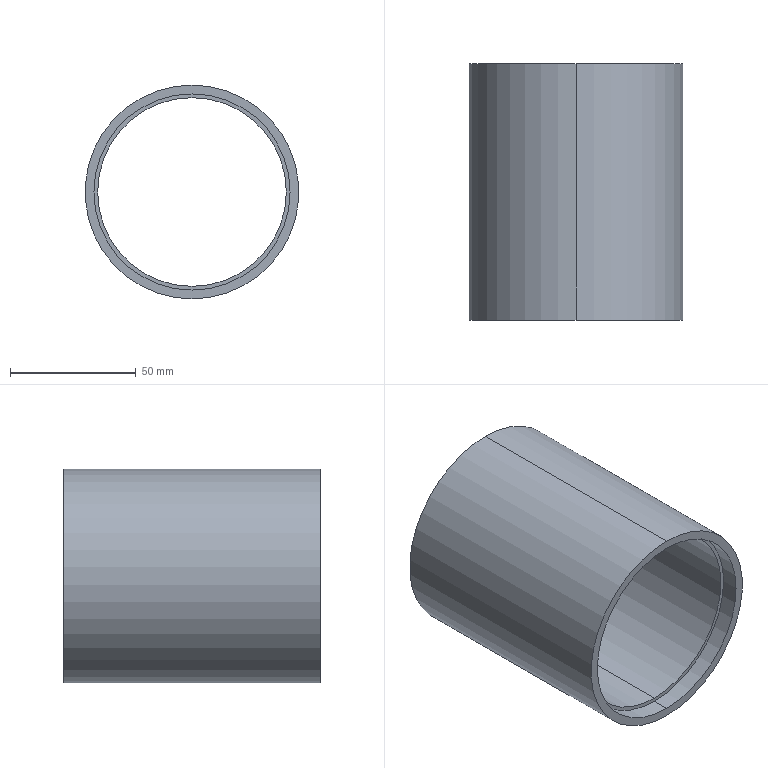Part | STEP file | 0229_Work-A | 1 solid | 11 faces | box 85 x 102 x 85 mm | volume 125379 mm3 | cylinder 6 | plane 3 | cone 2 | commonest cylinder face diameters 75 x2 78 x2 85 x2
STEP:
#1=CARTESIAN_POINT('',(0.,0.,0.));
#2=DIRECTION('',(0.,0.,1.));
#3=DIRECTION('',(1.,0.,0.));
#4=AXIS2_PLACEMENT_3D('',#1,#2,#3);
#5=CARTESIAN_POINT('',(0.,100.,37.5));
#6=VERTEX_POINT('',#5);
#7=CARTESIAN_POINT('',(0.,102.,38.655));
#8=VERTEX_POINT('',#7);
#9=CARTESIAN_POINT('',(0.,102.,38.655));
#10=DIRECTION('',(0.,0.866,0.5));
#11=VECTOR('',#10,1.);
#12=LINE('',#9,#11);
#13=CARTESIAN_POINT('',(0.,102.,0.));
#14=DIRECTION('',(0.,1.,0.));
#15=DIRECTION('',(0.,0.,1.));
#16=AXIS2_PLACEMENT_3D('',#13,#14,#15);
#17=CONICAL_SURFACE('',#16,38.655,0.5236);
#18=CARTESIAN_POINT('',(6.283,0.));
#19=DIRECTION('',(0.,1.));
#20=VECTOR('',#19,1.);
#21=LINE('',#18,#20);
#22=(GEOMETRIC_REPRESENTATION_CONTEXT(2)PARAMETRIC_REPRESENTATION_CONTEXT()REPRESENTATION_CONTEXT('',''));
#23=DEFINITIONAL_REPRESENTATION('',(#21),#22);
#24=PCURVE('',#17,#23);
#25=CARTESIAN_POINT('',(0.,102.,0.));
#26=DIRECTION('',(0.,1.,0.));
#27=DIRECTION('',(0.,0.,1.));
#28=AXIS2_PLACEMENT_3D('',#25,#26,#27);
#29=CONICAL_SURFACE('',#28,38.655,0.5236);
#30=CARTESIAN_POINT('',(0.,0.));
#31=DIRECTION('',(0.,1.));
#32=VECTOR('',#31,1.);
#33=LINE('',#30,#32);
#34=(GEOMETRIC_REPRESENTATION_CONTEXT(2)PARAMETRIC_REPRESENTATION_CONTEXT()REPRESENTATION_CONTEXT('',''));
#35=DEFINITIONAL_REPRESENTATION('',(#33),#34);
#36=PCURVE('',#29,#35);
#37=SURFACE_CURVE('',#12,(#24,#36),.PCURVE_S1.);
#38=EDGE_CURVE('',#6,#8,#37,.T.);
#39=ORIENTED_EDGE('',*,*,#38,.T.);
#40=CARTESIAN_POINT('',(0.,102.,-38.655));
#41=VERTEX_POINT('',#40);
#42=CARTESIAN_POINT('',(0.,102.,0.));
#43=DIRECTION('',(0.,-1.,0.));
#44=DIRECTION('',(0.,0.,-1.));
#45=AXIS2_PLACEMENT_3D('',#42,#43,#44);
#46=CIRCLE('',#45,38.655);
#47=CARTESIAN_POINT('',(9.425,0.));
#48=DIRECTION('',(-1.,0.));
#49=VECTOR('',#48,1.);
#50=LINE('',#47,#49);
#51=(GEOMETRIC_REPRESENTATION_CONTEXT(2)PARAMETRIC_REPRESENTATION_CONTEXT()REPRESENTATION_CONTEXT('',''));
#52=DEFINITIONAL_REPRESENTATION('',(#50),#51);
#53=PCURVE('',#17,#52);
#54=CARTESIAN_POINT('',(0.,102.,0.));
#55=DIRECTION('',(0.,-1.,0.));
#56=DIRECTION('',(0.,0.,-1.));
#57=AXIS2_PLACEMENT_3D('',#54,#55,#56);
#58=PLANE('',#57);
#59=CARTESIAN_POINT('',(0.,0.));
#60=DIRECTION('',(1.,0.));
#61=AXIS2_PLACEMENT_2D('',#59,#60);
#62=CIRCLE('',#61,38.655);
#63=(GEOMETRIC_REPRESENTATION_CONTEXT(2)PARAMETRIC_REPRESENTATION_CONTEXT()REPRESENTATION_CONTEXT('',''));
#64=DEFINITIONAL_REPRESENTATION('',(#62),#63);
#65=PCURVE('',#58,#64);
#66=SURFACE_CURVE('',#46,(#53,#65),.PCURVE_S1.);
#67=EDGE_CURVE('',#8,#41,#66,.T.);
#68=ORIENTED_EDGE('',*,*,#67,.T.);
#69=CARTESIAN_POINT('',(0.,100.,-37.5));
#70=VERTEX_POINT('',#69);
#71=CARTESIAN_POINT('',(0.,102.,-38.655));
#72=DIRECTION('',(0.,0.866,-0.5));
#73=VECTOR('',#72,1.);
#74=LINE('',#71,#73);
#75=CARTESIAN_POINT('',(3.142,0.));
#76=DIRECTION('',(0.,1.));
#77=VECTOR('',#76,1.);
#78=LINE('',#75,#77);
#79=(GEOMETRIC_REPRESENTATION_CONTEXT(2)PARAMETRIC_REPRESENTATION_CONTEXT()REPRESENTATION_CONTEXT('',''));
#80=DEFINITIONAL_REPRESENTATION('',(#78),#79);
#81=PCURVE('',#17,#80);
#82=CARTESIAN_POINT('',(3.142,0.));
#83=DIRECTION('',(0.,1.));
#84=VECTOR('',#83,1.);
#85=LINE('',#82,#84);
#86=(GEOMETRIC_REPRESENTATION_CONTEXT(2)PARAMETRIC_REPRESENTATION_CONTEXT()REPRESENTATION_CONTEXT('',''));
#87=DEFINITIONAL_REPRESENTATION('',(#85),#86);
#88=PCURVE('',#29,#87);
#89=SURFACE_CURVE('',#74,(#81,#88),.PCURVE_S1.);
#90=EDGE_CURVE('',#70,#41,#89,.T.);
#91=ORIENTED_EDGE('',*,*,#90,.F.);
#92=CARTESIAN_POINT('',(0.,100.,0.));
#93=DIRECTION('',(0.,1.,0.));
#94=DIRECTION('',(0.,0.,-1.));
#95=AXIS2_PLACEMENT_3D('',#92,#93,#94);
#96=CIRCLE('',#95,37.5);
#97=CARTESIAN_POINT('',(3.142,-2.));
#98=DIRECTION('',(1.,0.));
#99=VECTOR('',#98,1.);
#100=LINE('',#97,#99);
#101=(GEOMETRIC_REPRESENTATION_CONTEXT(2)PARAMETRIC_REPRESENTATION_CONTEXT()REPRESENTATION_CONTEXT('',''));
#102=DEFINITIONAL_REPRESENTATION('',(#100),#101);
#103=PCURVE('',#17,#102);
#104=CARTESIAN_POINT('',(0.,-11.457,0.));
#105=DIRECTION('',(0.,-1.,0.));
#106=DIRECTION('',(0.,0.,-1.));
#107=AXIS2_PLACEMENT_3D('',#104,#105,#106);
#108=CYLINDRICAL_SURFACE('',#107,37.5);
#109=CARTESIAN_POINT('',(6.283,-111.457));
#110=DIRECTION('',(-1.,0.));
#111=VECTOR('',#110,1.);
#112=LINE('',#109,#111);
#113=(GEOMETRIC_REPRESENTATION_CONTEXT(2)PARAMETRIC_REPRESENTATION_CONTEXT()REPRESENTATION_CONTEXT('',''));
#114=DEFINITIONAL_REPRESENTATION('',(#112),#113);
#115=PCURVE('',#108,#114);
#116=SURFACE_CURVE('',#96,(#103,#115),.PCURVE_S1.);
#117=EDGE_CURVE('',#70,#6,#116,.T.);
#118=ORIENTED_EDGE('',*,*,#117,.T.);
#119=EDGE_LOOP('',(#39,#68,#91,#118));
#120=FACE_BOUND('',#119,.F.);
#121=ADVANCED_FACE('',(#120),#17,.F.);
#122=CARTESIAN_POINT('',(0.,7.,-39.));
#123=VERTEX_POINT('',#122);
#124=CARTESIAN_POINT('',(0.,0.,-39.));
#125=VERTEX_POINT('',#124);
#126=CARTESIAN_POINT('',(0.,-11.457,-39.));
#127=DIRECTION('',(0.,-1.,0.));
#128=VECTOR('',#127,1.);
#129=LINE('',#126,#128);
#130=CARTESIAN_POINT('',(0.,-11.457,0.));
#131=DIRECTION('',(0.,-1.,0.));
#132=DIRECTION('',(0.,0.,-1.));
#133=AXIS2_PLACEMENT_3D('',#130,#131,#132);
#134=CYLINDRICAL_SURFACE('',#133,39.);
#135=CARTESIAN_POINT('',(6.283,0.));
#136=DIRECTION('',(0.,1.));
#137=VECTOR('',#136,1.);
#138=LINE('',#135,#137);
#139=(GEOMETRIC_REPRESENTATION_CONTEXT(2)PARAMETRIC_REPRESENTATION_CONTEXT()REPRESENTATION_CONTEXT('',''));
#140=DEFINITIONAL_REPRESENTATION('',(#138),#139);
#141=PCURVE('',#134,#140);
#142=CARTESIAN_POINT('',(0.,-11.457,0.));
#143=DIRECTION('',(0.,-1.,0.));
#144=DIRECTION('',(0.,0.,-1.));
#145=AXIS2_PLACEMENT_3D('',#142,#143,#144);
#146=CYLINDRICAL_SURFACE('',#145,39.);
#147=CARTESIAN_POINT('',(0.,0.));
#148=DIRECTION('',(0.,1.));
#149=VECTOR('',#148,1.);
#150=LINE('',#147,#149);
#151=(GEOMETRIC_REPRESENTATION_CONTEXT(2)PARAMETRIC_REPRESENTATION_CONTEXT()REPRESENTATION_CONTEXT('',''));
#152=DEFINITIONAL_REPRESENTATION('',(#150),#151);
#153=PCURVE('',#146,#152);
#154=SURFACE_CURVE('',#129,(#141,#153),.PCURVE_S1.);
#155=EDGE_CURVE('',#123,#125,#154,.T.);
#156=ORIENTED_EDGE('',*,*,#155,.T.);
#157=CARTESIAN_POINT('',(0.,0.,39.));
#158=VERTEX_POINT('',#157);
#159=CARTESIAN_POINT('',(0.,0.,0.));
#160=DIRECTION('',(0.,-1.,0.));
#161=DIRECTION('',(0.,0.,-1.));
#162=AXIS2_PLACEMENT_3D('',#159,#160,#161);
#163=CIRCLE('',#162,39.);
#164=CARTESIAN_POINT('',(0.,-11.457));
#165=DIRECTION('',(1.,0.));
#166=VECTOR('',#165,1.);
#167=LINE('',#164,#166);
#168=(GEOMETRIC_REPRESENTATION_CONTEXT(2)PARAMETRIC_REPRESENTATION_CONTEXT()REPRESENTATION_CONTEXT('',''));
#169=DEFINITIONAL_REPRESENTATION('',(#167),#168);
#170=PCURVE('',#134,#169);
#171=CARTESIAN_POINT('',(0.,0.,0.));
#172=DIRECTION('',(0.,1.,0.));
#173=DIRECTION('',(0.,0.,1.));
#174=AXIS2_PLACEMENT_3D('',#171,#172,#173);
#175=PLANE('',#174);
#176=CARTESIAN_POINT('',(-39.,0.));
#177=CARTESIAN_POINT('',(-39.,67.55));
#178=CARTESIAN_POINT('',(19.5,33.775));
#179=CARTESIAN_POINT('',(78.,0.));
#180=CARTESIAN_POINT('',(19.5,-33.775));
#181=CARTESIAN_POINT('',(-39.,-67.55));
#182=CARTESIAN_POINT('',(-39.,0.));
#183=(BOUNDED_CURVE()B_SPLINE_CURVE(2,(#176,#177,#178,#179,#180,#181,#182),.UNSPECIFIED.,.T.,.F.)B_SPLINE_CURVE_WITH_KNOTS((1,2,2,2,2,1),(-2.094,0.,2.094,4.189,6.283,8.378),.UNSPECIFIED.)CURVE()GEOMETRIC_REPRESENTATION_ITEM()RATIONAL_B_SPLINE_CURVE((1.,0.5,1.,0.5,1.,0.5,1.))REPRESENTATION_ITEM(''));
#184=(GEOMETRIC_REPRESENTATION_CONTEXT(2)PARAMETRIC_REPRESENTATION_CONTEXT()REPRESENTATION_CONTEXT('',''));
#185=DEFINITIONAL_REPRESENTATION('',(#183),#184);
#186=PCURVE('',#175,#185);
#187=SURFACE_CURVE('',#163,(#170,#186),.PCURVE_S1.);
#188=EDGE_CURVE('',#158,#125,#187,.T.);
#189=ORIENTED_EDGE('',*,*,#188,.F.);
#190=CARTESIAN_POINT('',(0.,7.,39.));
#191=VERTEX_POINT('',#190);
#192=CARTESIAN_POINT('',(0.,-11.457,39.));
#193=DIRECTION('',(0.,-1.,0.));
#194=VECTOR('',#193,1.);
#195=LINE('',#192,#194);
#196=CARTESIAN_POINT('',(3.142,0.));
#197=DIRECTION('',(0.,1.));
#198=VECTOR('',#197,1.);
#199=LINE('',#196,#198);
#200=(GEOMETRIC_REPRESENTATION_CONTEXT(2)PARAMETRIC_REPRESENTATION_CONTEXT()REPRESENTATION_CONTEXT('',''));
#201=DEFINITIONAL_REPRESENTATION('',(#199),#200);
#202=PCURVE('',#134,#201);
#203=CARTESIAN_POINT('',(3.142,0.));
#204=DIRECTION('',(0.,1.));
#205=VECTOR('',#204,1.);
#206=LINE('',#203,#205);
#207=(GEOMETRIC_REPRESENTATION_CONTEXT(2)PARAMETRIC_REPRESENTATION_CONTEXT()REPRESENTATION_CONTEXT('',''));
#208=DEFINITIONAL_REPRESENTATION('',(#206),#207);
#209=PCURVE('',#146,#208);
#210=SURFACE_CURVE('',#195,(#202,#209),.PCURVE_S1.);
#211=EDGE_CURVE('',#191,#158,#210,.T.);
#212=ORIENTED_EDGE('',*,*,#211,.F.);
#213=CARTESIAN_POINT('',(0.,7.,0.));
#214=DIRECTION('',(0.,-1.,0.));
#215=DIRECTION('',(0.,0.,-1.));
#216=AXIS2_PLACEMENT_3D('',#213,#214,#215);
#217=CIRCLE('',#216,39.);
#218=CARTESIAN_POINT('',(0.,-18.457));
#219=DIRECTION('',(1.,0.));
#220=VECTOR('',#219,1.);
#221=LINE('',#218,#220);
#222=(GEOMETRIC_REPRESENTATION_CONTEXT(2)PARAMETRIC_REPRESENTATION_CONTEXT()REPRESENTATION_CONTEXT('',''));
#223=DEFINITIONAL_REPRESENTATION('',(#221),#222);
#224=PCURVE('',#134,#223);
#225=CARTESIAN_POINT('',(-37.5,7.,0.));
#226=DIRECTION('',(0.,-1.,0.));
#227=DIRECTION('',(0.,0.,-1.));
#228=AXIS2_PLACEMENT_3D('',#225,#226,#227);
#229=PLANE('',#228);
#230=CARTESIAN_POINT('',(0.,37.5));
#231=DIRECTION('',(1.,0.));
#232=AXIS2_PLACEMENT_2D('',#230,#231);
#233=CIRCLE('',#232,39.);
#234=(GEOMETRIC_REPRESENTATION_CONTEXT(2)PARAMETRIC_REPRESENTATION_CONTEXT()REPRESENTATION_CONTEXT('',''));
#235=DEFINITIONAL_REPRESENTATION('',(#233),#234);
#236=PCURVE('',#229,#235);
#237=SURFACE_CURVE('',#217,(#224,#236),.PCURVE_S1.);
#238=EDGE_CURVE('',#191,#123,#237,.T.);
#239=ORIENTED_EDGE('',*,*,#238,.T.);
#240=EDGE_LOOP('',(#156,#189,#212,#239));
#241=FACE_BOUND('',#240,.F.);
#242=ADVANCED_FACE('',(#241),#134,.F.);
#243=CARTESIAN_POINT('',(0.,7.,-37.5));
#244=VERTEX_POINT('',#243);
#245=CARTESIAN_POINT('',(0.,-11.457,-37.5));
#246=DIRECTION('',(0.,-1.,0.));
#247=VECTOR('',#246,1.);
#248=LINE('',#245,#247);
#249=CARTESIAN_POINT('',(6.283,0.));
#250=DIRECTION('',(0.,1.));
#251=VECTOR('',#250,1.);
#252=LINE('',#249,#251);
#253=(GEOMETRIC_REPRESENTATION_CONTEXT(2)PARAMETRIC_REPRESENTATION_CONTEXT()REPRESENTATION_CONTEXT('',''));
#254=DEFINITIONAL_REPRESENTATION('',(#252),#253);
#255=PCURVE('',#108,#254);
#256=CARTESIAN_POINT('',(0.,-11.457,0.));
#257=DIRECTION('',(0.,-1.,0.));
#258=DIRECTION('',(0.,0.,-1.));
#259=AXIS2_PLACEMENT_3D('',#256,#257,#258);
#260=CYLINDRICAL_SURFACE('',#259,37.5);
#261=CARTESIAN_POINT('',(0.,0.));
#262=DIRECTION('',(0.,1.));
#263=VECTOR('',#262,1.);
#264=LINE('',#261,#263);
#265=(GEOMETRIC_REPRESENTATION_CONTEXT(2)PARAMETRIC_REPRESENTATION_CONTEXT()REPRESENTATION_CONTEXT('',''));
#266=DEFINITIONAL_REPRESENTATION('',(#264),#265);
#267=PCURVE('',#260,#266);
#268=SURFACE_CURVE('',#248,(#255,#267),.PCURVE_S1.);
#269=EDGE_CURVE('',#70,#244,#268,.T.);
#270=ORIENTED_EDGE('',*,*,#269,.T.);
#271=CARTESIAN_POINT('',(0.,7.,37.5));
#272=VERTEX_POINT('',#271);
#273=CARTESIAN_POINT('',(0.,7.,0.));
#274=DIRECTION('',(0.,-1.,0.));
#275=DIRECTION('',(0.,0.,-1.));
#276=AXIS2_PLACEMENT_3D('',#273,#274,#275);
#277=CIRCLE('',#276,37.5);
#278=CARTESIAN_POINT('',(0.,-18.457));
#279=DIRECTION('',(1.,0.));
#280=VECTOR('',#279,1.);
#281=LINE('',#278,#280);
#282=(GEOMETRIC_REPRESENTATION_CONTEXT(2)PARAMETRIC_REPRESENTATION_CONTEXT()REPRESENTATION_CONTEXT('',''));
#283=DEFINITIONAL_REPRESENTATION('',(#281),#282);
#284=PCURVE('',#108,#283);
#285=CARTESIAN_POINT('',(0.,37.5));
#286=DIRECTION('',(1.,0.));
#287=AXIS2_PLACEMENT_2D('',#285,#286);
#288=CIRCLE('',#287,37.5);
#289=(GEOMETRIC_REPRESENTATION_CONTEXT(2)PARAMETRIC_REPRESENTATION_CONTEXT()REPRESENTATION_CONTEXT('',''));
#290=DEFINITIONAL_REPRESENTATION('',(#288),#289);
#291=PCURVE('',#229,#290);
#292=SURFACE_CURVE('',#277,(#284,#291),.PCURVE_S1.);
#293=EDGE_CURVE('',#272,#244,#292,.T.);
#294=ORIENTED_EDGE('',*,*,#293,.F.);
#295=CARTESIAN_POINT('',(0.,-11.457,37.5));
#296=DIRECTION('',(0.,-1.,0.));
#297=VECTOR('',#296,1.);
#298=LINE('',#295,#297);
#299=CARTESIAN_POINT('',(3.142,0.));
#300=DIRECTION('',(0.,1.));
#301=VECTOR('',#300,1.);
#302=LINE('',#299,#301);
#303=(GEOMETRIC_REPRESENTATION_CONTEXT(2)PARAMETRIC_REPRESENTATION_CONTEXT()REPRESENTATION_CONTEXT('',''));
#304=DEFINITIONAL_REPRESENTATION('',(#302),#303);
#305=PCURVE('',#108,#304);
#306=CARTESIAN_POINT('',(3.142,0.));
#307=DIRECTION('',(0.,1.));
#308=VECTOR('',#307,1.);
#309=LINE('',#306,#308);
#310=(GEOMETRIC_REPRESENTATION_CONTEXT(2)PARAMETRIC_REPRESENTATION_CONTEXT()REPRESENTATION_CONTEXT('',''));
#311=DEFINITIONAL_REPRESENTATION('',(#309),#310);
#312=PCURVE('',#260,#311);
#313=SURFACE_CURVE('',#298,(#305,#312),.PCURVE_S1.);
#314=EDGE_CURVE('',#6,#272,#313,.T.);
#315=ORIENTED_EDGE('',*,*,#314,.F.);
#316=ORIENTED_EDGE('',*,*,#117,.F.);
#317=EDGE_LOOP('',(#270,#294,#315,#316));
#318=FACE_BOUND('',#317,.F.);
#319=ADVANCED_FACE('',(#318),#108,.F.);
#320=CARTESIAN_POINT('',(0.,102.,-42.5));
#321=VERTEX_POINT('',#320);
#322=CARTESIAN_POINT('',(0.,102.,42.5));
#323=VERTEX_POINT('',#322);
#324=CARTESIAN_POINT('',(0.,102.,0.));
#325=DIRECTION('',(0.,-1.,0.));
#326=DIRECTION('',(0.,0.,-1.));
#327=AXIS2_PLACEMENT_3D('',#324,#325,#326);
#328=CIRCLE('',#327,42.5);
#329=CARTESIAN_POINT('',(0.,-9.836,0.));
#330=DIRECTION('',(0.,-1.,0.));
#331=DIRECTION('',(0.,0.,-1.));
#332=AXIS2_PLACEMENT_3D('',#329,#330,#331);
#333=CYLINDRICAL_SURFACE('',#332,42.5);
#334=CARTESIAN_POINT('',(0.,-111.836));
#335=DIRECTION('',(1.,0.));
#336=VECTOR('',#335,1.);
#337=LINE('',#334,#336);
#338=(GEOMETRIC_REPRESENTATION_CONTEXT(2)PARAMETRIC_REPRESENTATION_CONTEXT()REPRESENTATION_CONTEXT('',''));
#339=DEFINITIONAL_REPRESENTATION('',(#337),#338);
#340=PCURVE('',#333,#339);
#341=CARTESIAN_POINT('',(0.,0.));
#342=DIRECTION('',(1.,0.));
#343=AXIS2_PLACEMENT_2D('',#341,#342);
#344=CIRCLE('',#343,42.5);
#345=(GEOMETRIC_REPRESENTATION_CONTEXT(2)PARAMETRIC_REPRESENTATION_CONTEXT()REPRESENTATION_CONTEXT('',''));
#346=DEFINITIONAL_REPRESENTATION('',(#344),#345);
#347=PCURVE('',#58,#346);
#348=SURFACE_CURVE('',#328,(#340,#347),.PCURVE_S1.);
#349=EDGE_CURVE('',#321,#323,#348,.T.);
#350=ORIENTED_EDGE('',*,*,#349,.T.);
#351=CARTESIAN_POINT('',(0.,0.,42.5));
#352=VERTEX_POINT('',#351);
#353=CARTESIAN_POINT('',(0.,-9.836,42.5));
#354=DIRECTION('',(0.,-1.,0.));
#355=VECTOR('',#354,1.);
#356=LINE('',#353,#355);
#357=CARTESIAN_POINT('',(3.142,0.));
#358=DIRECTION('',(0.,1.));
#359=VECTOR('',#358,1.);
#360=LINE('',#357,#359);
#361=(GEOMETRIC_REPRESENTATION_CONTEXT(2)PARAMETRIC_REPRESENTATION_CONTEXT()REPRESENTATION_CONTEXT('',''));
#362=DEFINITIONAL_REPRESENTATION('',(#360),#361);
#363=PCURVE('',#333,#362);
#364=CARTESIAN_POINT('',(0.,-9.836,0.));
#365=DIRECTION('',(0.,-1.,0.));
#366=DIRECTION('',(0.,0.,-1.));
#367=AXIS2_PLACEMENT_3D('',#364,#365,#366);
#368=CYLINDRICAL_SURFACE('',#367,42.5);
#369=CARTESIAN_POINT('',(3.142,0.));
#370=DIRECTION('',(0.,1.));
#371=VECTOR('',#370,1.);
#372=LINE('',#369,#371);
#373=(GEOMETRIC_REPRESENTATION_CONTEXT(2)PARAMETRIC_REPRESENTATION_CONTEXT()REPRESENTATION_CONTEXT('',''));
#374=DEFINITIONAL_REPRESENTATION('',(#372),#373);
#375=PCURVE('',#368,#374);
#376=SURFACE_CURVE('',#356,(#363,#375),.PCURVE_S1.);
#377=EDGE_CURVE('',#323,#352,#376,.T.);
#378=ORIENTED_EDGE('',*,*,#377,.T.);
#379=CARTESIAN_POINT('',(0.,0.,-42.5));
#380=VERTEX_POINT('',#379);
#381=CARTESIAN_POINT('',(0.,0.,0.));
#382=DIRECTION('',(0.,-1.,0.));
#383=DIRECTION('',(0.,0.,-1.));
#384=AXIS2_PLACEMENT_3D('',#381,#382,#383);
#385=CIRCLE('',#384,42.5);
#386=CARTESIAN_POINT('',(0.,-9.836));
#387=DIRECTION('',(1.,0.));
#388=VECTOR('',#387,1.);
#389=LINE('',#386,#388);
#390=(GEOMETRIC_REPRESENTATION_CONTEXT(2)PARAMETRIC_REPRESENTATION_CONTEXT()REPRESENTATION_CONTEXT('',''));
#391=DEFINITIONAL_REPRESENTATION('',(#389),#390);
#392=PCURVE('',#333,#391);
#393=CARTESIAN_POINT('',(-42.5,0.));
#394=CARTESIAN_POINT('',(-42.5,73.612));
#395=CARTESIAN_POINT('',(21.25,36.806));
#396=CARTESIAN_POINT('',(85.,0.));
#397=CARTESIAN_POINT('',(21.25,-36.806));
#398=CARTESIAN_POINT('',(-42.5,-73.612));
#399=CARTESIAN_POINT('',(-42.5,0.));
#400=(BOUNDED_CURVE()B_SPLINE_CURVE(2,(#393,#394,#395,#396,#397,#398,#399),.UNSPECIFIED.,.T.,.F.)B_SPLINE_CURVE_WITH_KNOTS((1,2,2,2,2,1),(-2.094,0.,2.094,4.189,6.283,8.378),.UNSPECIFIED.)CURVE()GEOMETRIC_REPRESENTATION_ITEM()RATIONAL_B_SPLINE_CURVE((1.,0.5,1.,0.5,1.,0.5,1.))REPRESENTATION_ITEM(''));
#401=(GEOMETRIC_REPRESENTATION_CONTEXT(2)PARAMETRIC_REPRESENTATION_CONTEXT()REPRESENTATION_CONTEXT('',''));
#402=DEFINITIONAL_REPRESENTATION('',(#400),#401);
#403=PCURVE('',#175,#402);
#404=SURFACE_CURVE('',#385,(#392,#403),.PCURVE_S1.);
#405=EDGE_CURVE('',#380,#352,#404,.T.);
#406=ORIENTED_EDGE('',*,*,#405,.F.);
#407=CARTESIAN_POINT('',(0.,-9.836,-42.5));
#408=DIRECTION('',(0.,-1.,0.));
#409=VECTOR('',#408,1.);
#410=LINE('',#407,#409);
#411=CARTESIAN_POINT('',(0.,0.));
#412=DIRECTION('',(0.,1.));
#413=VECTOR('',#412,1.);
#414=LINE('',#411,#413);
#415=(GEOMETRIC_REPRESENTATION_CONTEXT(2)PARAMETRIC_REPRESENTATION_CONTEXT()REPRESENTATION_CONTEXT('',''));
#416=DEFINITIONAL_REPRESENTATION('',(#414),#415);
#417=PCURVE('',#333,#416);
#418=CARTESIAN_POINT('',(6.283,0.));
#419=DIRECTION('',(0.,1.));
#420=VECTOR('',#419,1.);
#421=LINE('',#418,#420);
#422=(GEOMETRIC_REPRESENTATION_CONTEXT(2)PARAMETRIC_REPRESENTATION_CONTEXT()REPRESENTATION_CONTEXT('',''));
#423=DEFINITIONAL_REPRESENTATION('',(#421),#422);
#424=PCURVE('',#368,#423);
#425=SURFACE_CURVE('',#410,(#417,#424),.PCURVE_S1.);
#426=EDGE_CURVE('',#321,#380,#425,.T.);
#427=ORIENTED_EDGE('',*,*,#426,.F.);
#428=EDGE_LOOP('',(#350,#378,#406,#427));
#429=FACE_BOUND('',#428,.T.);
#430=ADVANCED_FACE('',(#429),#333,.T.);
#431=ORIENTED_EDGE('',*,*,#67,.T.);
#432=CARTESIAN_POINT('',(0.,102.,0.));
#433=DIRECTION('',(0.,-1.,0.));
#434=DIRECTION('',(0.,0.,-1.));
#435=AXIS2_PLACEMENT_3D('',#432,#433,#434);
#436=CIRCLE('',#435,38.655);
#437=CARTESIAN_POINT('',(0.,0.));
#438=DIRECTION('',(1.,0.));
#439=AXIS2_PLACEMENT_2D('',#437,#438);
#440=CIRCLE('',#439,38.655);
#441=(GEOMETRIC_REPRESENTATION_CONTEXT(2)PARAMETRIC_REPRESENTATION_CONTEXT()REPRESENTATION_CONTEXT('',''));
#442=DEFINITIONAL_REPRESENTATION('',(#440),#441);
#443=PCURVE('',#58,#442);
#444=CARTESIAN_POINT('',(3.142,0.));
#445=DIRECTION('',(-1.,0.));
#446=VECTOR('',#445,1.);
#447=LINE('',#444,#446);
#448=(GEOMETRIC_REPRESENTATION_CONTEXT(2)PARAMETRIC_REPRESENTATION_CONTEXT()REPRESENTATION_CONTEXT('',''));
#449=DEFINITIONAL_REPRESENTATION('',(#447),#448);
#450=PCURVE('',#29,#449);
#451=SURFACE_CURVE('',#436,(#443,#450),.PCURVE_S1.);
#452=EDGE_CURVE('',#41,#8,#451,.T.);
#453=ORIENTED_EDGE('',*,*,#452,.T.);
#454=EDGE_LOOP('',(#431,#453));
#455=FACE_BOUND('',#454,.T.);
#456=ORIENTED_EDGE('',*,*,#349,.F.);
#457=CARTESIAN_POINT('',(0.,102.,0.));
#458=DIRECTION('',(0.,-1.,0.));
#459=DIRECTION('',(0.,0.,-1.));
#460=AXIS2_PLACEMENT_3D('',#457,#458,#459);
#461=CIRCLE('',#460,42.5);
#462=CARTESIAN_POINT('',(0.,0.));
#463=DIRECTION('',(1.,0.));
#464=AXIS2_PLACEMENT_2D('',#462,#463);
#465=CIRCLE('',#464,42.5);
#466=(GEOMETRIC_REPRESENTATION_CONTEXT(2)PARAMETRIC_REPRESENTATION_CONTEXT()REPRESENTATION_CONTEXT('',''));
#467=DEFINITIONAL_REPRESENTATION('',(#465),#466);
#468=PCURVE('',#58,#467);
#469=CARTESIAN_POINT('',(0.,-111.836));
#470=DIRECTION('',(1.,0.));
#471=VECTOR('',#470,1.);
#472=LINE('',#469,#471);
#473=(GEOMETRIC_REPRESENTATION_CONTEXT(2)PARAMETRIC_REPRESENTATION_CONTEXT()REPRESENTATION_CONTEXT('',''));
#474=DEFINITIONAL_REPRESENTATION('',(#472),#473);
#475=PCURVE('',#368,#474);
#476=SURFACE_CURVE('',#461,(#468,#475),.PCURVE_S1.);
#477=EDGE_CURVE('',#323,#321,#476,.T.);
#478=ORIENTED_EDGE('',*,*,#477,.F.);
#479=EDGE_LOOP('',(#456,#478));
#480=FACE_BOUND('',#479,.T.);
#481=ADVANCED_FACE('',(#455,#480),#58,.F.);
#482=ORIENTED_EDGE('',*,*,#405,.T.);
#483=CARTESIAN_POINT('',(0.,0.,0.));
#484=DIRECTION('',(0.,-1.,0.));
#485=DIRECTION('',(0.,0.,-1.));
#486=AXIS2_PLACEMENT_3D('',#483,#484,#485);
#487=CIRCLE('',#486,42.5);
#488=CARTESIAN_POINT('',(-42.5,0.));
#489=CARTESIAN_POINT('',(-42.5,73.612));
#490=CARTESIAN_POINT('',(21.25,36.806));
#491=CARTESIAN_POINT('',(85.,0.));
#492=CARTESIAN_POINT('',(21.25,-36.806));
#493=CARTESIAN_POINT('',(-42.5,-73.612));
#494=CARTESIAN_POINT('',(-42.5,0.));
#495=(BOUNDED_CURVE()B_SPLINE_CURVE(2,(#488,#489,#490,#491,#492,#493,#494),.UNSPECIFIED.,.T.,.F.)B_SPLINE_CURVE_WITH_KNOTS((1,2,2,2,2,1),(-2.094,0.,2.094,4.189,6.283,8.378),.UNSPECIFIED.)CURVE()GEOMETRIC_REPRESENTATION_ITEM()RATIONAL_B_SPLINE_CURVE((1.,0.5,1.,0.5,1.,0.5,1.))REPRESENTATION_ITEM(''));
#496=(GEOMETRIC_REPRESENTATION_CONTEXT(2)PARAMETRIC_REPRESENTATION_CONTEXT()REPRESENTATION_CONTEXT('',''));
#497=DEFINITIONAL_REPRESENTATION('',(#495),#496);
#498=PCURVE('',#175,#497);
#499=CARTESIAN_POINT('',(0.,-9.836));
#500=DIRECTION('',(1.,0.));
#501=VECTOR('',#500,1.);
#502=LINE('',#499,#501);
#503=(GEOMETRIC_REPRESENTATION_CONTEXT(2)PARAMETRIC_REPRESENTATION_CONTEXT()REPRESENTATION_CONTEXT('',''));
#504=DEFINITIONAL_REPRESENTATION('',(#502),#503);
#505=PCURVE('',#368,#504);
#506=SURFACE_CURVE('',#487,(#498,#505),.PCURVE_S1.);
#507=EDGE_CURVE('',#352,#380,#506,.T.);
#508=ORIENTED_EDGE('',*,*,#507,.T.);
#509=EDGE_LOOP('',(#482,#508));
#510=FACE_BOUND('',#509,.T.);
#511=CARTESIAN_POINT('',(0.,0.,0.));
#512=DIRECTION('',(0.,-1.,0.));
#513=DIRECTION('',(0.,0.,-1.));
#514=AXIS2_PLACEMENT_3D('',#511,#512,#513);
#515=CIRCLE('',#514,39.);
#516=CARTESIAN_POINT('',(-39.,0.));
#517=CARTESIAN_POINT('',(-39.,67.55));
#518=CARTESIAN_POINT('',(19.5,33.775));
#519=CARTESIAN_POINT('',(78.,0.));
#520=CARTESIAN_POINT('',(19.5,-33.775));
#521=CARTESIAN_POINT('',(-39.,-67.55));
#522=CARTESIAN_POINT('',(-39.,0.));
#523=(BOUNDED_CURVE()B_SPLINE_CURVE(2,(#516,#517,#518,#519,#520,#521,#522),.UNSPECIFIED.,.T.,.F.)B_SPLINE_CURVE_WITH_KNOTS((1,2,2,2,2,1),(-2.094,0.,2.094,4.189,6.283,8.378),.UNSPECIFIED.)CURVE()GEOMETRIC_REPRESENTATION_ITEM()RATIONAL_B_SPLINE_CURVE((1.,0.5,1.,0.5,1.,0.5,1.))REPRESENTATION_ITEM(''));
#524=(GEOMETRIC_REPRESENTATION_CONTEXT(2)PARAMETRIC_REPRESENTATION_CONTEXT()REPRESENTATION_CONTEXT('',''));
#525=DEFINITIONAL_REPRESENTATION('',(#523),#524);
#526=PCURVE('',#175,#525);
#527=CARTESIAN_POINT('',(0.,-11.457));
#528=DIRECTION('',(1.,0.));
#529=VECTOR('',#528,1.);
#530=LINE('',#527,#529);
#531=(GEOMETRIC_REPRESENTATION_CONTEXT(2)PARAMETRIC_REPRESENTATION_CONTEXT()REPRESENTATION_CONTEXT('',''));
#532=DEFINITIONAL_REPRESENTATION('',(#530),#531);
#533=PCURVE('',#146,#532);
#534=SURFACE_CURVE('',#515,(#526,#533),.PCURVE_S1.);
#535=EDGE_CURVE('',#125,#158,#534,.T.);
#536=ORIENTED_EDGE('',*,*,#535,.F.);
#537=ORIENTED_EDGE('',*,*,#188,.F.);
#538=EDGE_LOOP('',(#536,#537));
#539=FACE_BOUND('',#538,.T.);
#540=ADVANCED_FACE('',(#510,#539),#175,.F.);
#541=ORIENTED_EDGE('',*,*,#377,.F.);
#542=ORIENTED_EDGE('',*,*,#477,.T.);
#543=ORIENTED_EDGE('',*,*,#426,.T.);
#544=ORIENTED_EDGE('',*,*,#507,.F.);
#545=EDGE_LOOP('',(#541,#542,#543,#544));
#546=FACE_BOUND('',#545,.T.);
#547=ADVANCED_FACE('',(#546),#368,.T.);
#548=CARTESIAN_POINT('',(0.,7.,0.));
#549=DIRECTION('',(0.,-1.,0.));
#550=DIRECTION('',(0.,0.,-1.));
#551=AXIS2_PLACEMENT_3D('',#548,#549,#550);
#552=CIRCLE('',#551,37.5);
#553=CARTESIAN_POINT('',(0.,-18.457));
#554=DIRECTION('',(1.,0.));
#555=VECTOR('',#554,1.);
#556=LINE('',#553,#555);
#557=(GEOMETRIC_REPRESENTATION_CONTEXT(2)PARAMETRIC_REPRESENTATION_CONTEXT()REPRESENTATION_CONTEXT('',''));
#558=DEFINITIONAL_REPRESENTATION('',(#556),#557);
#559=PCURVE('',#260,#558);
#560=CARTESIAN_POINT('',(0.,37.5));
#561=DIRECTION('',(1.,0.));
#562=AXIS2_PLACEMENT_2D('',#560,#561);
#563=CIRCLE('',#562,37.5);
#564=(GEOMETRIC_REPRESENTATION_CONTEXT(2)PARAMETRIC_REPRESENTATION_CONTEXT()REPRESENTATION_CONTEXT('',''));
#565=DEFINITIONAL_REPRESENTATION('',(#563),#564);
#566=PCURVE('',#229,#565);
#567=SURFACE_CURVE('',#552,(#559,#566),.PCURVE_S1.);
#568=EDGE_CURVE('',#244,#272,#567,.T.);
#569=ORIENTED_EDGE('',*,*,#568,.F.);
#570=ORIENTED_EDGE('',*,*,#269,.F.);
#571=CARTESIAN_POINT('',(0.,100.,0.));
#572=DIRECTION('',(0.,1.,0.));
#573=DIRECTION('',(0.,0.,-1.));
#574=AXIS2_PLACEMENT_3D('',#571,#572,#573);
#575=CIRCLE('',#574,37.5);
#576=CARTESIAN_POINT('',(6.283,-111.457));
#577=DIRECTION('',(-1.,0.));
#578=VECTOR('',#577,1.);
#579=LINE('',#576,#578);
#580=(GEOMETRIC_REPRESENTATION_CONTEXT(2)PARAMETRIC_REPRESENTATION_CONTEXT()REPRESENTATION_CONTEXT('',''));
#581=DEFINITIONAL_REPRESENTATION('',(#579),#580);
#582=PCURVE('',#260,#581);
#583=CARTESIAN_POINT('',(-3.142,-2.));
#584=DIRECTION('',(1.,0.));
#585=VECTOR('',#584,1.);
#586=LINE('',#583,#585);
#587=(GEOMETRIC_REPRESENTATION_CONTEXT(2)PARAMETRIC_REPRESENTATION_CONTEXT()REPRESENTATION_CONTEXT('',''));
#588=DEFINITIONAL_REPRESENTATION('',(#586),#587);
#589=PCURVE('',#29,#588);
#590=SURFACE_CURVE('',#575,(#582,#589),.PCURVE_S1.);
#591=EDGE_CURVE('',#6,#70,#590,.T.);
#592=ORIENTED_EDGE('',*,*,#591,.F.);
#593=ORIENTED_EDGE('',*,*,#314,.T.);
#594=EDGE_LOOP('',(#569,#570,#592,#593));
#595=FACE_BOUND('',#594,.F.);
#596=ADVANCED_FACE('',(#595),#260,.F.);
#597=CARTESIAN_POINT('',(0.,7.,0.));
#598=DIRECTION('',(0.,-1.,0.));
#599=DIRECTION('',(0.,0.,-1.));
#600=AXIS2_PLACEMENT_3D('',#597,#598,#599);
#601=CIRCLE('',#600,39.);
#602=CARTESIAN_POINT('',(0.,37.5));
#603=DIRECTION('',(1.,0.));
#604=AXIS2_PLACEMENT_2D('',#602,#603);
#605=CIRCLE('',#604,39.);
#606=(GEOMETRIC_REPRESENTATION_CONTEXT(2)PARAMETRIC_REPRESENTATION_CONTEXT()REPRESENTATION_CONTEXT('',''));
#607=DEFINITIONAL_REPRESENTATION('',(#605),#606);
#608=PCURVE('',#229,#607);
#609=CARTESIAN_POINT('',(0.,-18.457));
#610=DIRECTION('',(1.,0.));
#611=VECTOR('',#610,1.);
#612=LINE('',#609,#611);
#613=(GEOMETRIC_REPRESENTATION_CONTEXT(2)PARAMETRIC_REPRESENTATION_CONTEXT()REPRESENTATION_CONTEXT('',''));
#614=DEFINITIONAL_REPRESENTATION('',(#612),#613);
#615=PCURVE('',#146,#614);
#616=SURFACE_CURVE('',#601,(#608,#615),.PCURVE_S1.);
#617=EDGE_CURVE('',#123,#191,#616,.T.);
#618=ORIENTED_EDGE('',*,*,#617,.T.);
#619=ORIENTED_EDGE('',*,*,#238,.T.);
#620=EDGE_LOOP('',(#618,#619));
#621=FACE_BOUND('',#620,.T.);
#622=ORIENTED_EDGE('',*,*,#568,.F.);
#623=ORIENTED_EDGE('',*,*,#293,.F.);
#624=EDGE_LOOP('',(#622,#623));
#625=FACE_BOUND('',#624,.T.);
#626=ADVANCED_FACE('',(#621,#625),#229,.T.);
#627=ORIENTED_EDGE('',*,*,#535,.F.);
#628=ORIENTED_EDGE('',*,*,#155,.F.);
#629=ORIENTED_EDGE('',*,*,#617,.T.);
#630=ORIENTED_EDGE('',*,*,#211,.T.);
#631=EDGE_LOOP('',(#627,#628,#629,#630));
#632=FACE_BOUND('',#631,.F.);
#633=ADVANCED_FACE('',(#632),#146,.F.);
#634=ORIENTED_EDGE('',*,*,#452,.T.);
#635=ORIENTED_EDGE('',*,*,#38,.F.);
#636=ORIENTED_EDGE('',*,*,#591,.T.);
#637=ORIENTED_EDGE('',*,*,#90,.T.);
#638=EDGE_LOOP('',(#634,#635,#636,#637));
#639=FACE_BOUND('',#638,.F.);
#640=ADVANCED_FACE('',(#639),#29,.F.);
#641=CLOSED_SHELL('',(#121,#242,#319,#430,#481,#540,#547,#596,#626,#633,#640));
#642=MANIFOLD_SOLID_BREP('',#641);
#643=(LENGTH_UNIT()NAMED_UNIT(*)SI_UNIT(.MILLI.,.METRE.));
#644=UNCERTAINTY_MEASURE_WITH_UNIT(LENGTH_MEASURE(0.0000001),#643,'','');
#645=(NAMED_UNIT(*)PLANE_ANGLE_UNIT()SI_UNIT($,.RADIAN.));
#646=(NAMED_UNIT(*)SI_UNIT($,.STERADIAN.)SOLID_ANGLE_UNIT());
#647=(GEOMETRIC_REPRESENTATION_CONTEXT(3)GLOBAL_UNCERTAINTY_ASSIGNED_CONTEXT((#644))GLOBAL_UNIT_ASSIGNED_CONTEXT((#643,#645,#646))REPRESENTATION_CONTEXT('',''));
#648=ADVANCED_BREP_SHAPE_REPRESENTATION('',(#4,#642),#647);